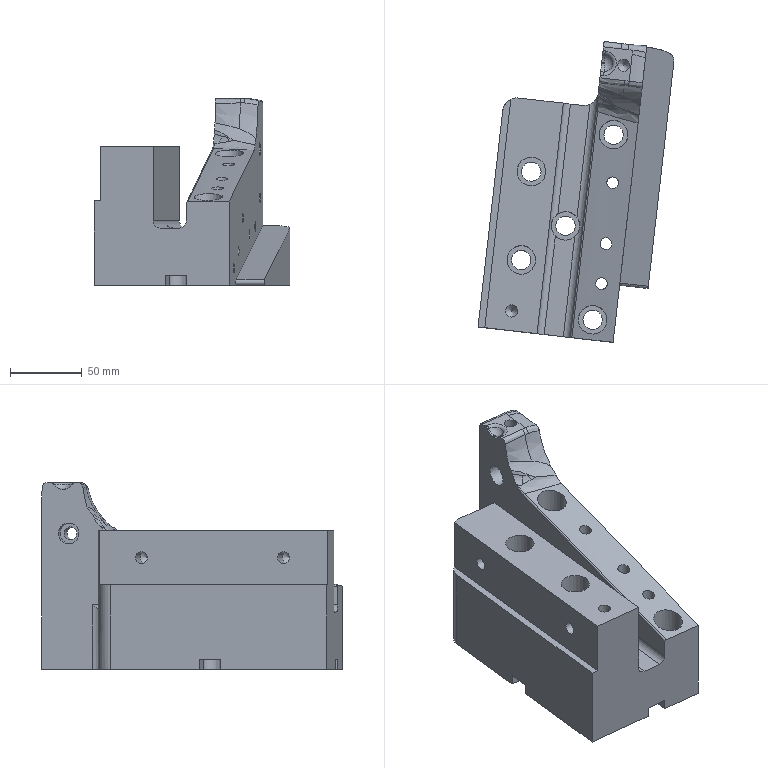Part | NX | features 23 2 | 1 solid | 112 faces | box 136.979 x 210.262 x 130.4 mm | volume 1259749 mm3 | cylinder 42 | plane 38 | spline 16 | cone 10 | torus 6 | commonest cylinder face diameters 20 x7 6.8 x6 13.5 x5 8.5 x4 7 x3 8.2 x3